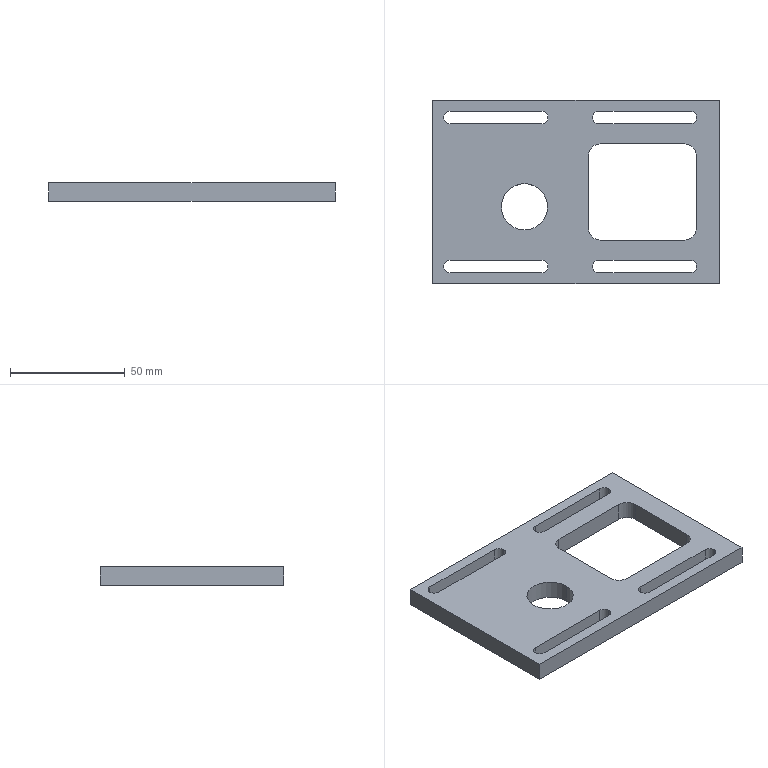Part | STEP file | rotary cylinder plate | 1 solid | 40 faces | box 125 x 80 x 8 mm | volume 54016 mm3 | cylinder 22 | plane 18 | commonest cylinder face diameters 5.5 x16 10 x4 20.2 x2